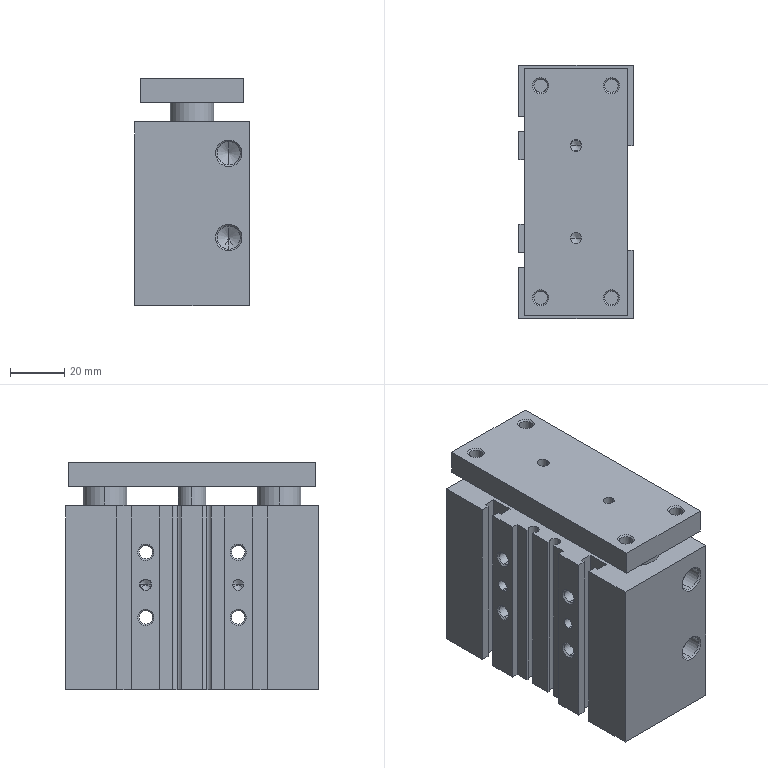Part | SolidWorks | 2 solids | 234 faces | box 42 x 93 x 83.5 mm | volume 253192 mm3 | cylinder 88 | plane 78 | cone 68 | commonest cylinder face diameters 4.917 x24 4 x18 5.4 x8 8.566 x8 9.5 x8 16 x8